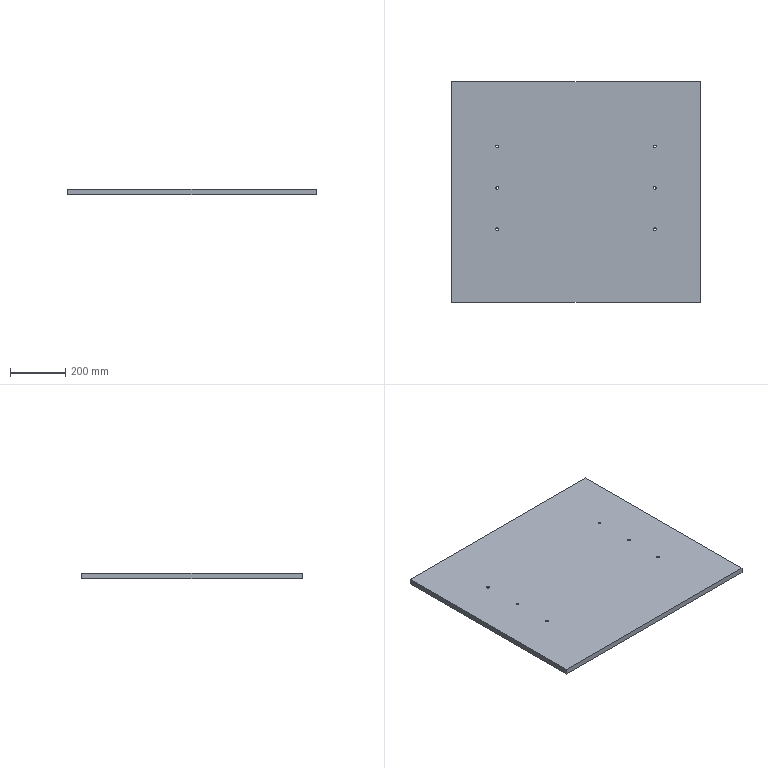Part | SolidWorks | features BaseBody 1 | 1 solid | 18 faces | box 900 x 800 x 20 mm | volume 14390194 mm3 | cylinder 12 | plane 6 | commonest cylinder face diameters 10.2 x12
STEP:
#1=CARTESIAN_POINT('',(285.,170.1,10.));
#2=VERTEX_POINT('',#1);
#3=CARTESIAN_POINT('',(285.,159.9,10.));
#4=VERTEX_POINT('',#3);
#5=CARTESIAN_POINT('',(285.,165.,10.));
#6=DIRECTION('',(0.,0.,1.));
#7=DIRECTION('',(0.,1.,0.));
#8=AXIS2_PLACEMENT_3D('',#5,#6,#7);
#9=CIRCLE('',#8,5.1);
#10=EDGE_CURVE('',#2,#4,#9,.T.);
#11=ORIENTED_EDGE('',*,*,#10,.T.);
#12=CARTESIAN_POINT('',(285.,159.9,-10.));
#13=VERTEX_POINT('',#12);
#14=CARTESIAN_POINT('',(285.,159.9,10.));
#15=DIRECTION('',(0.,0.,-1.));
#16=VECTOR('',#15,1000.);
#17=LINE('',#14,#16);
#18=EDGE_CURVE('',#4,#13,#17,.T.);
#19=ORIENTED_EDGE('',*,*,#18,.T.);
#20=CARTESIAN_POINT('',(285.,170.1,-10.));
#21=VERTEX_POINT('',#20);
#22=CARTESIAN_POINT('',(285.,165.,-10.));
#23=DIRECTION('',(0.,0.,-1.));
#24=DIRECTION('',(0.,1.,0.));
#25=AXIS2_PLACEMENT_3D('',#22,#23,#24);
#26=CIRCLE('',#25,5.1);
#27=EDGE_CURVE('',#13,#21,#26,.T.);
#28=ORIENTED_EDGE('',*,*,#27,.T.);
#29=CARTESIAN_POINT('',(285.,170.1,10.));
#30=DIRECTION('',(0.,0.,-1.));
#31=VECTOR('',#30,1000.);
#32=LINE('',#29,#31);
#33=EDGE_CURVE('',#2,#21,#32,.T.);
#34=ORIENTED_EDGE('',*,*,#33,.F.);
#35=EDGE_LOOP('',(#11,#19,#28,#34));
#36=FACE_OUTER_BOUND('',#35,.T.);
#37=CARTESIAN_POINT('',(285.,165.,10.));
#38=DIRECTION('',(0.,0.,-1.));
#39=DIRECTION('',(0.,1.,0.));
#40=AXIS2_PLACEMENT_3D('',#37,#38,#39);
#41=CYLINDRICAL_SURFACE('',#40,5.1);
#42=ADVANCED_FACE('',(#36),#41,.F.);
#43=CARTESIAN_POINT('',(-285.,170.1,10.));
#44=VERTEX_POINT('',#43);
#45=CARTESIAN_POINT('',(-285.,159.9,10.));
#46=VERTEX_POINT('',#45);
#47=CARTESIAN_POINT('',(-285.,165.,10.));
#48=DIRECTION('',(0.,0.,1.));
#49=DIRECTION('',(0.,1.,0.));
#50=AXIS2_PLACEMENT_3D('',#47,#48,#49);
#51=CIRCLE('',#50,5.1);
#52=EDGE_CURVE('',#44,#46,#51,.T.);
#53=ORIENTED_EDGE('',*,*,#52,.T.);
#54=CARTESIAN_POINT('',(-285.,159.9,-10.));
#55=VERTEX_POINT('',#54);
#56=CARTESIAN_POINT('',(-285.,159.9,10.));
#57=DIRECTION('',(0.,0.,-1.));
#58=VECTOR('',#57,1000.);
#59=LINE('',#56,#58);
#60=EDGE_CURVE('',#46,#55,#59,.T.);
#61=ORIENTED_EDGE('',*,*,#60,.T.);
#62=CARTESIAN_POINT('',(-285.,170.1,-10.));
#63=VERTEX_POINT('',#62);
#64=CARTESIAN_POINT('',(-285.,165.,-10.));
#65=DIRECTION('',(0.,0.,1.));
#66=DIRECTION('',(0.,1.,0.));
#67=AXIS2_PLACEMENT_3D('',#64,#65,#66);
#68=CIRCLE('',#67,5.1);
#69=EDGE_CURVE('',#63,#55,#68,.T.);
#70=ORIENTED_EDGE('',*,*,#69,.F.);
#71=CARTESIAN_POINT('',(-285.,170.1,10.));
#72=DIRECTION('',(0.,0.,-1.));
#73=VECTOR('',#72,1000.);
#74=LINE('',#71,#73);
#75=EDGE_CURVE('',#44,#63,#74,.T.);
#76=ORIENTED_EDGE('',*,*,#75,.F.);
#77=EDGE_LOOP('',(#53,#61,#70,#76));
#78=FACE_OUTER_BOUND('',#77,.T.);
#79=CARTESIAN_POINT('',(-285.,165.,10.));
#80=DIRECTION('',(0.,0.,-1.));
#81=DIRECTION('',(0.,1.,0.));
#82=AXIS2_PLACEMENT_3D('',#79,#80,#81);
#83=CYLINDRICAL_SURFACE('',#82,5.1);
#84=ADVANCED_FACE('',(#78),#83,.F.);
#85=CARTESIAN_POINT('',(-285.,20.1,10.));
#86=VERTEX_POINT('',#85);
#87=CARTESIAN_POINT('',(-285.,9.9,10.));
#88=VERTEX_POINT('',#87);
#89=CARTESIAN_POINT('',(-285.,15.,10.));
#90=DIRECTION('',(0.,0.,1.));
#91=DIRECTION('',(0.,1.,0.));
#92=AXIS2_PLACEMENT_3D('',#89,#90,#91);
#93=CIRCLE('',#92,5.1);
#94=EDGE_CURVE('',#86,#88,#93,.T.);
#95=ORIENTED_EDGE('',*,*,#94,.T.);
#96=CARTESIAN_POINT('',(-285.,9.9,-10.));
#97=VERTEX_POINT('',#96);
#98=CARTESIAN_POINT('',(-285.,9.9,10.));
#99=DIRECTION('',(0.,0.,-1.));
#100=VECTOR('',#99,1000.);
#101=LINE('',#98,#100);
#102=EDGE_CURVE('',#88,#97,#101,.T.);
#103=ORIENTED_EDGE('',*,*,#102,.T.);
#104=CARTESIAN_POINT('',(-285.,20.1,-10.));
#105=VERTEX_POINT('',#104);
#106=CARTESIAN_POINT('',(-285.,15.,-10.));
#107=DIRECTION('',(0.,0.,1.));
#108=DIRECTION('',(0.,1.,0.));
#109=AXIS2_PLACEMENT_3D('',#106,#107,#108);
#110=CIRCLE('',#109,5.1);
#111=EDGE_CURVE('',#105,#97,#110,.T.);
#112=ORIENTED_EDGE('',*,*,#111,.F.);
#113=CARTESIAN_POINT('',(-285.,20.1,10.));
#114=DIRECTION('',(0.,0.,-1.));
#115=VECTOR('',#114,1000.);
#116=LINE('',#113,#115);
#117=EDGE_CURVE('',#86,#105,#116,.T.);
#118=ORIENTED_EDGE('',*,*,#117,.F.);
#119=EDGE_LOOP('',(#95,#103,#112,#118));
#120=FACE_OUTER_BOUND('',#119,.T.);
#121=CARTESIAN_POINT('',(-285.,15.,10.));
#122=DIRECTION('',(0.,0.,-1.));
#123=DIRECTION('',(0.,1.,0.));
#124=AXIS2_PLACEMENT_3D('',#121,#122,#123);
#125=CYLINDRICAL_SURFACE('',#124,5.1);
#126=ADVANCED_FACE('',(#120),#125,.F.);
#127=CARTESIAN_POINT('',(-285.,-129.9,10.));
#128=VERTEX_POINT('',#127);
#129=CARTESIAN_POINT('',(-285.,-140.1,10.));
#130=VERTEX_POINT('',#129);
#131=CARTESIAN_POINT('',(-285.,-135.,10.));
#132=DIRECTION('',(0.,0.,1.));
#133=DIRECTION('',(0.,1.,0.));
#134=AXIS2_PLACEMENT_3D('',#131,#132,#133);
#135=CIRCLE('',#134,5.1);
#136=EDGE_CURVE('',#128,#130,#135,.T.);
#137=ORIENTED_EDGE('',*,*,#136,.T.);
#138=CARTESIAN_POINT('',(-285.,-140.1,-10.));
#139=VERTEX_POINT('',#138);
#140=CARTESIAN_POINT('',(-285.,-140.1,10.));
#141=DIRECTION('',(0.,0.,-1.));
#142=VECTOR('',#141,1000.);
#143=LINE('',#140,#142);
#144=EDGE_CURVE('',#130,#139,#143,.T.);
#145=ORIENTED_EDGE('',*,*,#144,.T.);
#146=CARTESIAN_POINT('',(-285.,-129.9,-10.));
#147=VERTEX_POINT('',#146);
#148=CARTESIAN_POINT('',(-285.,-135.,-10.));
#149=DIRECTION('',(0.,0.,1.));
#150=DIRECTION('',(0.,1.,0.));
#151=AXIS2_PLACEMENT_3D('',#148,#149,#150);
#152=CIRCLE('',#151,5.1);
#153=EDGE_CURVE('',#147,#139,#152,.T.);
#154=ORIENTED_EDGE('',*,*,#153,.F.);
#155=CARTESIAN_POINT('',(-285.,-129.9,10.));
#156=DIRECTION('',(0.,0.,-1.));
#157=VECTOR('',#156,1000.);
#158=LINE('',#155,#157);
#159=EDGE_CURVE('',#128,#147,#158,.T.);
#160=ORIENTED_EDGE('',*,*,#159,.F.);
#161=EDGE_LOOP('',(#137,#145,#154,#160));
#162=FACE_OUTER_BOUND('',#161,.T.);
#163=CARTESIAN_POINT('',(-285.,-135.,10.));
#164=DIRECTION('',(0.,0.,-1.));
#165=DIRECTION('',(0.,1.,0.));
#166=AXIS2_PLACEMENT_3D('',#163,#164,#165);
#167=CYLINDRICAL_SURFACE('',#166,5.1);
#168=ADVANCED_FACE('',(#162),#167,.F.);
#169=CARTESIAN_POINT('',(285.,-129.9,10.));
#170=VERTEX_POINT('',#169);
#171=CARTESIAN_POINT('',(285.,-140.1,10.));
#172=VERTEX_POINT('',#171);
#173=CARTESIAN_POINT('',(285.,-135.,10.));
#174=DIRECTION('',(0.,0.,1.));
#175=DIRECTION('',(0.,1.,0.));
#176=AXIS2_PLACEMENT_3D('',#173,#174,#175);
#177=CIRCLE('',#176,5.1);
#178=EDGE_CURVE('',#170,#172,#177,.T.);
#179=ORIENTED_EDGE('',*,*,#178,.T.);
#180=CARTESIAN_POINT('',(285.,-140.1,-10.));
#181=VERTEX_POINT('',#180);
#182=CARTESIAN_POINT('',(285.,-140.1,10.));
#183=DIRECTION('',(0.,0.,-1.));
#184=VECTOR('',#183,1000.);
#185=LINE('',#182,#184);
#186=EDGE_CURVE('',#172,#181,#185,.T.);
#187=ORIENTED_EDGE('',*,*,#186,.T.);
#188=CARTESIAN_POINT('',(285.,-129.9,-10.));
#189=VERTEX_POINT('',#188);
#190=CARTESIAN_POINT('',(285.,-135.,-10.));
#191=DIRECTION('',(0.,0.,1.));
#192=DIRECTION('',(0.,1.,0.));
#193=AXIS2_PLACEMENT_3D('',#190,#191,#192);
#194=CIRCLE('',#193,5.1);
#195=EDGE_CURVE('',#189,#181,#194,.T.);
#196=ORIENTED_EDGE('',*,*,#195,.F.);
#197=CARTESIAN_POINT('',(285.,-129.9,10.));
#198=DIRECTION('',(0.,0.,-1.));
#199=VECTOR('',#198,1000.);
#200=LINE('',#197,#199);
#201=EDGE_CURVE('',#170,#189,#200,.T.);
#202=ORIENTED_EDGE('',*,*,#201,.F.);
#203=EDGE_LOOP('',(#179,#187,#196,#202));
#204=FACE_OUTER_BOUND('',#203,.T.);
#205=CARTESIAN_POINT('',(285.,-135.,10.));
#206=DIRECTION('',(0.,0.,-1.));
#207=DIRECTION('',(0.,1.,0.));
#208=AXIS2_PLACEMENT_3D('',#205,#206,#207);
#209=CYLINDRICAL_SURFACE('',#208,5.1);
#210=ADVANCED_FACE('',(#204),#209,.F.);
#211=CARTESIAN_POINT('',(285.,20.1,10.));
#212=VERTEX_POINT('',#211);
#213=CARTESIAN_POINT('',(285.,9.9,10.));
#214=VERTEX_POINT('',#213);
#215=CARTESIAN_POINT('',(285.,15.,10.));
#216=DIRECTION('',(0.,0.,1.));
#217=DIRECTION('',(0.,1.,0.));
#218=AXIS2_PLACEMENT_3D('',#215,#216,#217);
#219=CIRCLE('',#218,5.1);
#220=EDGE_CURVE('',#212,#214,#219,.T.);
#221=ORIENTED_EDGE('',*,*,#220,.T.);
#222=CARTESIAN_POINT('',(285.,9.9,-10.));
#223=VERTEX_POINT('',#222);
#224=CARTESIAN_POINT('',(285.,9.9,10.));
#225=DIRECTION('',(0.,0.,-1.));
#226=VECTOR('',#225,1000.);
#227=LINE('',#224,#226);
#228=EDGE_CURVE('',#214,#223,#227,.T.);
#229=ORIENTED_EDGE('',*,*,#228,.T.);
#230=CARTESIAN_POINT('',(285.,20.1,-10.));
#231=VERTEX_POINT('',#230);
#232=CARTESIAN_POINT('',(285.,15.,-10.));
#233=DIRECTION('',(0.,0.,1.));
#234=DIRECTION('',(0.,1.,0.));
#235=AXIS2_PLACEMENT_3D('',#232,#233,#234);
#236=CIRCLE('',#235,5.1);
#237=EDGE_CURVE('',#231,#223,#236,.T.);
#238=ORIENTED_EDGE('',*,*,#237,.F.);
#239=CARTESIAN_POINT('',(285.,20.1,10.));
#240=DIRECTION('',(0.,0.,-1.));
#241=VECTOR('',#240,1000.);
#242=LINE('',#239,#241);
#243=EDGE_CURVE('',#212,#231,#242,.T.);
#244=ORIENTED_EDGE('',*,*,#243,.F.);
#245=EDGE_LOOP('',(#221,#229,#238,#244));
#246=FACE_OUTER_BOUND('',#245,.T.);
#247=CARTESIAN_POINT('',(285.,15.,10.));
#248=DIRECTION('',(0.,0.,-1.));
#249=DIRECTION('',(0.,1.,0.));
#250=AXIS2_PLACEMENT_3D('',#247,#248,#249);
#251=CYLINDRICAL_SURFACE('',#250,5.1);
#252=ADVANCED_FACE('',(#246),#251,.F.);
#253=ORIENTED_EDGE('',*,*,#18,.F.);
#254=CARTESIAN_POINT('',(285.,165.,10.));
#255=DIRECTION('',(0.,0.,1.));
#256=DIRECTION('',(0.,1.,0.));
#257=AXIS2_PLACEMENT_3D('',#254,#255,#256);
#258=CIRCLE('',#257,5.1);
#259=EDGE_CURVE('',#4,#2,#258,.T.);
#260=ORIENTED_EDGE('',*,*,#259,.T.);
#261=ORIENTED_EDGE('',*,*,#33,.T.);
#262=CARTESIAN_POINT('',(285.,165.,-10.));
#263=DIRECTION('',(0.,0.,-1.));
#264=DIRECTION('',(0.,1.,0.));
#265=AXIS2_PLACEMENT_3D('',#262,#263,#264);
#266=CIRCLE('',#265,5.1);
#267=EDGE_CURVE('',#21,#13,#266,.T.);
#268=ORIENTED_EDGE('',*,*,#267,.T.);
#269=EDGE_LOOP('',(#253,#260,#261,#268));
#270=FACE_OUTER_BOUND('',#269,.T.);
#271=CARTESIAN_POINT('',(285.,165.,10.));
#272=DIRECTION('',(0.,0.,-1.));
#273=DIRECTION('',(0.,1.,0.));
#274=AXIS2_PLACEMENT_3D('',#271,#272,#273);
#275=CYLINDRICAL_SURFACE('',#274,5.1);
#276=ADVANCED_FACE('',(#270),#275,.F.);
#277=ORIENTED_EDGE('',*,*,#69,.T.);
#278=CARTESIAN_POINT('',(-285.,165.,-10.));
#279=DIRECTION('',(0.,0.,1.));
#280=DIRECTION('',(0.,1.,0.));
#281=AXIS2_PLACEMENT_3D('',#278,#279,#280);
#282=CIRCLE('',#281,5.1);
#283=EDGE_CURVE('',#55,#63,#282,.T.);
#284=ORIENTED_EDGE('',*,*,#283,.T.);
#285=EDGE_LOOP('',(#277,#284));
#286=FACE_BOUND('',#285,.T.);
#287=ORIENTED_EDGE('',*,*,#111,.T.);
#288=CARTESIAN_POINT('',(-285.,15.,-10.));
#289=DIRECTION('',(0.,0.,1.));
#290=DIRECTION('',(0.,1.,0.));
#291=AXIS2_PLACEMENT_3D('',#288,#289,#290);
#292=CIRCLE('',#291,5.1);
#293=EDGE_CURVE('',#97,#105,#292,.T.);
#294=ORIENTED_EDGE('',*,*,#293,.T.);
#295=EDGE_LOOP('',(#287,#294));
#296=FACE_BOUND('',#295,.T.);
#297=ORIENTED_EDGE('',*,*,#153,.T.);
#298=CARTESIAN_POINT('',(-285.,-135.,-10.));
#299=DIRECTION('',(0.,0.,1.));
#300=DIRECTION('',(0.,1.,0.));
#301=AXIS2_PLACEMENT_3D('',#298,#299,#300);
#302=CIRCLE('',#301,5.1);
#303=EDGE_CURVE('',#139,#147,#302,.T.);
#304=ORIENTED_EDGE('',*,*,#303,.T.);
#305=EDGE_LOOP('',(#297,#304));
#306=FACE_BOUND('',#305,.T.);
#307=ORIENTED_EDGE('',*,*,#195,.T.);
#308=CARTESIAN_POINT('',(285.,-135.,-10.));
#309=DIRECTION('',(0.,0.,1.));
#310=DIRECTION('',(0.,1.,0.));
#311=AXIS2_PLACEMENT_3D('',#308,#309,#310);
#312=CIRCLE('',#311,5.1);
#313=EDGE_CURVE('',#181,#189,#312,.T.);
#314=ORIENTED_EDGE('',*,*,#313,.T.);
#315=EDGE_LOOP('',(#307,#314));
#316=FACE_BOUND('',#315,.T.);
#317=ORIENTED_EDGE('',*,*,#237,.T.);
#318=CARTESIAN_POINT('',(285.,15.,-10.));
#319=DIRECTION('',(0.,0.,1.));
#320=DIRECTION('',(0.,1.,0.));
#321=AXIS2_PLACEMENT_3D('',#318,#319,#320);
#322=CIRCLE('',#321,5.1);
#323=EDGE_CURVE('',#223,#231,#322,.T.);
#324=ORIENTED_EDGE('',*,*,#323,.T.);
#325=EDGE_LOOP('',(#317,#324));
#326=FACE_BOUND('',#325,.T.);
#327=ORIENTED_EDGE('',*,*,#267,.F.);
#328=ORIENTED_EDGE('',*,*,#27,.F.);
#329=EDGE_LOOP('',(#327,#328));
#330=FACE_BOUND('',#329,.T.);
#331=CARTESIAN_POINT('',(-450.,-400.,-10.));
#332=VERTEX_POINT('',#331);
#333=CARTESIAN_POINT('',(-450.,400.,-10.));
#334=VERTEX_POINT('',#333);
#335=CARTESIAN_POINT('',(-450.,0.,-10.));
#336=DIRECTION('',(0.,1.,0.));
#337=VECTOR('',#336,1000.);
#338=LINE('',#335,#337);
#339=EDGE_CURVE('',#332,#334,#338,.T.);
#340=ORIENTED_EDGE('',*,*,#339,.T.);
#341=CARTESIAN_POINT('',(450.,400.,-10.));
#342=VERTEX_POINT('',#341);
#343=CARTESIAN_POINT('',(0.,400.,-10.));
#344=DIRECTION('',(1.,0.,0.));
#345=VECTOR('',#344,1000.);
#346=LINE('',#343,#345);
#347=EDGE_CURVE('',#334,#342,#346,.T.);
#348=ORIENTED_EDGE('',*,*,#347,.T.);
#349=CARTESIAN_POINT('',(450.,-400.,-10.));
#350=VERTEX_POINT('',#349);
#351=CARTESIAN_POINT('',(450.,0.,-10.));
#352=DIRECTION('',(0.,-1.,0.));
#353=VECTOR('',#352,1000.);
#354=LINE('',#351,#353);
#355=EDGE_CURVE('',#342,#350,#354,.T.);
#356=ORIENTED_EDGE('',*,*,#355,.T.);
#357=CARTESIAN_POINT('',(0.,-400.,-10.));
#358=DIRECTION('',(-1.,0.,0.));
#359=VECTOR('',#358,1000.);
#360=LINE('',#357,#359);
#361=EDGE_CURVE('',#350,#332,#360,.T.);
#362=ORIENTED_EDGE('',*,*,#361,.T.);
#363=EDGE_LOOP('',(#340,#348,#356,#362));
#364=FACE_OUTER_BOUND('',#363,.T.);
#365=CARTESIAN_POINT('',(450.,-400.,-10.));
#366=DIRECTION('',(0.,0.,-1.));
#367=DIRECTION('',(-1.,0.,0.));
#368=AXIS2_PLACEMENT_3D('',#365,#366,#367);
#369=PLANE('',#368);
#370=ADVANCED_FACE('',(#286,#296,#306,#316,#326,#330,#364),#369,.T.);
#371=ORIENTED_EDGE('',*,*,#52,.F.);
#372=CARTESIAN_POINT('',(-285.,165.,10.));
#373=DIRECTION('',(0.,0.,1.));
#374=DIRECTION('',(0.,1.,0.));
#375=AXIS2_PLACEMENT_3D('',#372,#373,#374);
#376=CIRCLE('',#375,5.1);
#377=EDGE_CURVE('',#46,#44,#376,.T.);
#378=ORIENTED_EDGE('',*,*,#377,.F.);
#379=EDGE_LOOP('',(#371,#378));
#380=FACE_BOUND('',#379,.T.);
#381=ORIENTED_EDGE('',*,*,#94,.F.);
#382=CARTESIAN_POINT('',(-285.,15.,10.));
#383=DIRECTION('',(0.,0.,1.));
#384=DIRECTION('',(0.,1.,0.));
#385=AXIS2_PLACEMENT_3D('',#382,#383,#384);
#386=CIRCLE('',#385,5.1);
#387=EDGE_CURVE('',#88,#86,#386,.T.);
#388=ORIENTED_EDGE('',*,*,#387,.F.);
#389=EDGE_LOOP('',(#381,#388));
#390=FACE_BOUND('',#389,.T.);
#391=ORIENTED_EDGE('',*,*,#136,.F.);
#392=CARTESIAN_POINT('',(-285.,-135.,10.));
#393=DIRECTION('',(0.,0.,1.));
#394=DIRECTION('',(0.,1.,0.));
#395=AXIS2_PLACEMENT_3D('',#392,#393,#394);
#396=CIRCLE('',#395,5.1);
#397=EDGE_CURVE('',#130,#128,#396,.T.);
#398=ORIENTED_EDGE('',*,*,#397,.F.);
#399=EDGE_LOOP('',(#391,#398));
#400=FACE_BOUND('',#399,.T.);
#401=ORIENTED_EDGE('',*,*,#178,.F.);
#402=CARTESIAN_POINT('',(285.,-135.,10.));
#403=DIRECTION('',(0.,0.,1.));
#404=DIRECTION('',(0.,1.,0.));
#405=AXIS2_PLACEMENT_3D('',#402,#403,#404);
#406=CIRCLE('',#405,5.1);
#407=EDGE_CURVE('',#172,#170,#406,.T.);
#408=ORIENTED_EDGE('',*,*,#407,.F.);
#409=EDGE_LOOP('',(#401,#408));
#410=FACE_BOUND('',#409,.T.);
#411=ORIENTED_EDGE('',*,*,#220,.F.);
#412=CARTESIAN_POINT('',(285.,15.,10.));
#413=DIRECTION('',(0.,0.,1.));
#414=DIRECTION('',(0.,1.,0.));
#415=AXIS2_PLACEMENT_3D('',#412,#413,#414);
#416=CIRCLE('',#415,5.1);
#417=EDGE_CURVE('',#214,#212,#416,.T.);
#418=ORIENTED_EDGE('',*,*,#417,.F.);
#419=EDGE_LOOP('',(#411,#418));
#420=FACE_BOUND('',#419,.T.);
#421=ORIENTED_EDGE('',*,*,#10,.F.);
#422=ORIENTED_EDGE('',*,*,#259,.F.);
#423=EDGE_LOOP('',(#421,#422));
#424=FACE_BOUND('',#423,.T.);
#425=CARTESIAN_POINT('',(-450.,400.,10.));
#426=VERTEX_POINT('',#425);
#427=CARTESIAN_POINT('',(450.,400.,10.));
#428=VERTEX_POINT('',#427);
#429=CARTESIAN_POINT('',(0.,400.,10.));
#430=DIRECTION('',(1.,0.,0.));
#431=VECTOR('',#430,1000.);
#432=LINE('',#429,#431);
#433=EDGE_CURVE('',#426,#428,#432,.T.);
#434=ORIENTED_EDGE('',*,*,#433,.F.);
#435=CARTESIAN_POINT('',(-450.,-400.,10.));
#436=VERTEX_POINT('',#435);
#437=CARTESIAN_POINT('',(-450.,0.,10.));
#438=DIRECTION('',(0.,1.,0.));
#439=VECTOR('',#438,1000.);
#440=LINE('',#437,#439);
#441=EDGE_CURVE('',#436,#426,#440,.T.);
#442=ORIENTED_EDGE('',*,*,#441,.F.);
#443=CARTESIAN_POINT('',(450.,-400.,10.));
#444=VERTEX_POINT('',#443);
#445=CARTESIAN_POINT('',(0.,-400.,10.));
#446=DIRECTION('',(-1.,0.,0.));
#447=VECTOR('',#446,1000.);
#448=LINE('',#445,#447);
#449=EDGE_CURVE('',#444,#436,#448,.T.);
#450=ORIENTED_EDGE('',*,*,#449,.F.);
#451=CARTESIAN_POINT('',(450.,0.,10.));
#452=DIRECTION('',(0.,-1.,0.));
#453=VECTOR('',#452,1000.);
#454=LINE('',#451,#453);
#455=EDGE_CURVE('',#428,#444,#454,.T.);
#456=ORIENTED_EDGE('',*,*,#455,.F.);
#457=EDGE_LOOP('',(#434,#442,#450,#456));
#458=FACE_OUTER_BOUND('',#457,.T.);
#459=CARTESIAN_POINT('',(450.,-400.,10.));
#460=DIRECTION('',(0.,0.,-1.));
#461=DIRECTION('',(-1.,0.,0.));
#462=AXIS2_PLACEMENT_3D('',#459,#460,#461);
#463=PLANE('',#462);
#464=ADVANCED_FACE('',(#380,#390,#400,#410,#420,#424,#458),#463,.F.);
#465=ORIENTED_EDGE('',*,*,#60,.F.);
#466=ORIENTED_EDGE('',*,*,#377,.T.);
#467=ORIENTED_EDGE('',*,*,#75,.T.);
#468=ORIENTED_EDGE('',*,*,#283,.F.);
#469=EDGE_LOOP('',(#465,#466,#467,#468));
#470=FACE_OUTER_BOUND('',#469,.T.);
#471=CARTESIAN_POINT('',(-285.,165.,10.));
#472=DIRECTION('',(0.,0.,-1.));
#473=DIRECTION('',(0.,1.,0.));
#474=AXIS2_PLACEMENT_3D('',#471,#472,#473);
#475=CYLINDRICAL_SURFACE('',#474,5.1);
#476=ADVANCED_FACE('',(#470),#475,.F.);
#477=ORIENTED_EDGE('',*,*,#102,.F.);
#478=ORIENTED_EDGE('',*,*,#387,.T.);
#479=ORIENTED_EDGE('',*,*,#117,.T.);
#480=ORIENTED_EDGE('',*,*,#293,.F.);
#481=EDGE_LOOP('',(#477,#478,#479,#480));
#482=FACE_OUTER_BOUND('',#481,.T.);
#483=CARTESIAN_POINT('',(-285.,15.,10.));
#484=DIRECTION('',(0.,0.,-1.));
#485=DIRECTION('',(0.,1.,0.));
#486=AXIS2_PLACEMENT_3D('',#483,#484,#485);
#487=CYLINDRICAL_SURFACE('',#486,5.1);
#488=ADVANCED_FACE('',(#482),#487,.F.);
#489=ORIENTED_EDGE('',*,*,#144,.F.);
#490=ORIENTED_EDGE('',*,*,#397,.T.);
#491=ORIENTED_EDGE('',*,*,#159,.T.);
#492=ORIENTED_EDGE('',*,*,#303,.F.);
#493=EDGE_LOOP('',(#489,#490,#491,#492));
#494=FACE_OUTER_BOUND('',#493,.T.);
#495=CARTESIAN_POINT('',(-285.,-135.,10.));
#496=DIRECTION('',(0.,0.,-1.));
#497=DIRECTION('',(0.,1.,0.));
#498=AXIS2_PLACEMENT_3D('',#495,#496,#497);
#499=CYLINDRICAL_SURFACE('',#498,5.1);
#500=ADVANCED_FACE('',(#494),#499,.F.);
#501=ORIENTED_EDGE('',*,*,#186,.F.);
#502=ORIENTED_EDGE('',*,*,#407,.T.);
#503=ORIENTED_EDGE('',*,*,#201,.T.);
#504=ORIENTED_EDGE('',*,*,#313,.F.);
#505=EDGE_LOOP('',(#501,#502,#503,#504));
#506=FACE_OUTER_BOUND('',#505,.T.);
#507=CARTESIAN_POINT('',(285.,-135.,10.));
#508=DIRECTION('',(0.,0.,-1.));
#509=DIRECTION('',(0.,1.,0.));
#510=AXIS2_PLACEMENT_3D('',#507,#508,#509);
#511=CYLINDRICAL_SURFACE('',#510,5.1);
#512=ADVANCED_FACE('',(#506),#511,.F.);
#513=ORIENTED_EDGE('',*,*,#228,.F.);
#514=ORIENTED_EDGE('',*,*,#417,.T.);
#515=ORIENTED_EDGE('',*,*,#243,.T.);
#516=ORIENTED_EDGE('',*,*,#323,.F.);
#517=EDGE_LOOP('',(#513,#514,#515,#516));
#518=FACE_OUTER_BOUND('',#517,.T.);
#519=CARTESIAN_POINT('',(285.,15.,10.));
#520=DIRECTION('',(0.,0.,-1.));
#521=DIRECTION('',(0.,1.,0.));
#522=AXIS2_PLACEMENT_3D('',#519,#520,#521);
#523=CYLINDRICAL_SURFACE('',#522,5.1);
#524=ADVANCED_FACE('',(#518),#523,.F.);
#525=CARTESIAN_POINT('',(-450.,400.,0.));
#526=DIRECTION('',(0.,0.,-1.));
#527=VECTOR('',#526,1000.);
#528=LINE('',#525,#527);
#529=EDGE_CURVE('',#426,#334,#528,.T.);
#530=ORIENTED_EDGE('',*,*,#529,.F.);
#531=ORIENTED_EDGE('',*,*,#433,.T.);
#532=CARTESIAN_POINT('',(450.,400.,0.));
#533=DIRECTION('',(0.,0.,1.));
#534=VECTOR('',#533,1000.);
#535=LINE('',#532,#534);
#536=EDGE_CURVE('',#342,#428,#535,.T.);
#537=ORIENTED_EDGE('',*,*,#536,.F.);
#538=ORIENTED_EDGE('',*,*,#347,.F.);
#539=EDGE_LOOP('',(#530,#531,#537,#538));
#540=FACE_OUTER_BOUND('',#539,.T.);
#541=CARTESIAN_POINT('',(-450.,400.,10.));
#542=DIRECTION('',(0.,-1.,0.));
#543=DIRECTION('',(0.,0.,-1.));
#544=AXIS2_PLACEMENT_3D('',#541,#542,#543);
#545=PLANE('',#544);
#546=ADVANCED_FACE('',(#540),#545,.F.);
#547=CARTESIAN_POINT('',(-450.,-400.,0.));
#548=DIRECTION('',(0.,0.,-1.));
#549=VECTOR('',#548,1000.);
#550=LINE('',#547,#549);
#551=EDGE_CURVE('',#436,#332,#550,.T.);
#552=ORIENTED_EDGE('',*,*,#551,.F.);
#553=ORIENTED_EDGE('',*,*,#441,.T.);
#554=ORIENTED_EDGE('',*,*,#529,.T.);
#555=ORIENTED_EDGE('',*,*,#339,.F.);
#556=EDGE_LOOP('',(#552,#553,#554,#555));
#557=FACE_OUTER_BOUND('',#556,.T.);
#558=CARTESIAN_POINT('',(-450.,-400.,10.));
#559=DIRECTION('',(1.,0.,0.));
#560=DIRECTION('',(0.,0.,-1.));
#561=AXIS2_PLACEMENT_3D('',#558,#559,#560);
#562=PLANE('',#561);
#563=ADVANCED_FACE('',(#557),#562,.F.);
#564=CARTESIAN_POINT('',(450.,-400.,0.));
#565=DIRECTION('',(0.,0.,-1.));
#566=VECTOR('',#565,1000.);
#567=LINE('',#564,#566);
#568=EDGE_CURVE('',#444,#350,#567,.T.);
#569=ORIENTED_EDGE('',*,*,#568,.F.);
#570=ORIENTED_EDGE('',*,*,#449,.T.);
#571=ORIENTED_EDGE('',*,*,#551,.T.);
#572=ORIENTED_EDGE('',*,*,#361,.F.);
#573=EDGE_LOOP('',(#569,#570,#571,#572));
#574=FACE_OUTER_BOUND('',#573,.T.);
#575=CARTESIAN_POINT('',(-450.,-400.,-10.));
#576=DIRECTION('',(0.,1.,0.));
#577=DIRECTION('',(0.,0.,1.));
#578=AXIS2_PLACEMENT_3D('',#575,#576,#577);
#579=PLANE('',#578);
#580=ADVANCED_FACE('',(#574),#579,.F.);
#581=ORIENTED_EDGE('',*,*,#536,.T.);
#582=ORIENTED_EDGE('',*,*,#455,.T.);
#583=ORIENTED_EDGE('',*,*,#568,.T.);
#584=ORIENTED_EDGE('',*,*,#355,.F.);
#585=EDGE_LOOP('',(#581,#582,#583,#584));
#586=FACE_OUTER_BOUND('',#585,.T.);
#587=CARTESIAN_POINT('',(450.,-400.,-10.));
#588=DIRECTION('',(-1.,0.,0.));
#589=DIRECTION('',(0.,0.,1.));
#590=AXIS2_PLACEMENT_3D('',#587,#588,#589);
#591=PLANE('',#590);
#592=ADVANCED_FACE('',(#586),#591,.F.);
#593=CLOSED_SHELL('',(#42,#84,#126,#168,#210,#252,#276,#370,#464,#476,#488,#500,#512,#524,#546,#563,#580,#592));
#594=MANIFOLD_SOLID_BREP('',#593);
#595=CARTESIAN_POINT('',(0.,0.,0.));
#596=DIRECTION('',(0.,0.,1.));
#597=DIRECTION('',(1.,0.,0.));
#598=AXIS2_PLACEMENT_3D('',#595,#596,#597);
#599=(LENGTH_UNIT()NAMED_UNIT(*)SI_UNIT(.MILLI.,.METRE.));
#600=UNCERTAINTY_MEASURE_WITH_UNIT(LENGTH_MEASURE(0.00001),#599,'','');
#601=(NAMED_UNIT(*)PLANE_ANGLE_UNIT()SI_UNIT($,.RADIAN.));
#602=(NAMED_UNIT(*)SI_UNIT($,.STERADIAN.)SOLID_ANGLE_UNIT());
#603=(GEOMETRIC_REPRESENTATION_CONTEXT(3)GLOBAL_UNCERTAINTY_ASSIGNED_CONTEXT((#600))GLOBAL_UNIT_ASSIGNED_CONTEXT((#599,#601,#602))REPRESENTATION_CONTEXT('',''));
#604=ADVANCED_BREP_SHAPE_REPRESENTATION('',(#594,#598),#603);